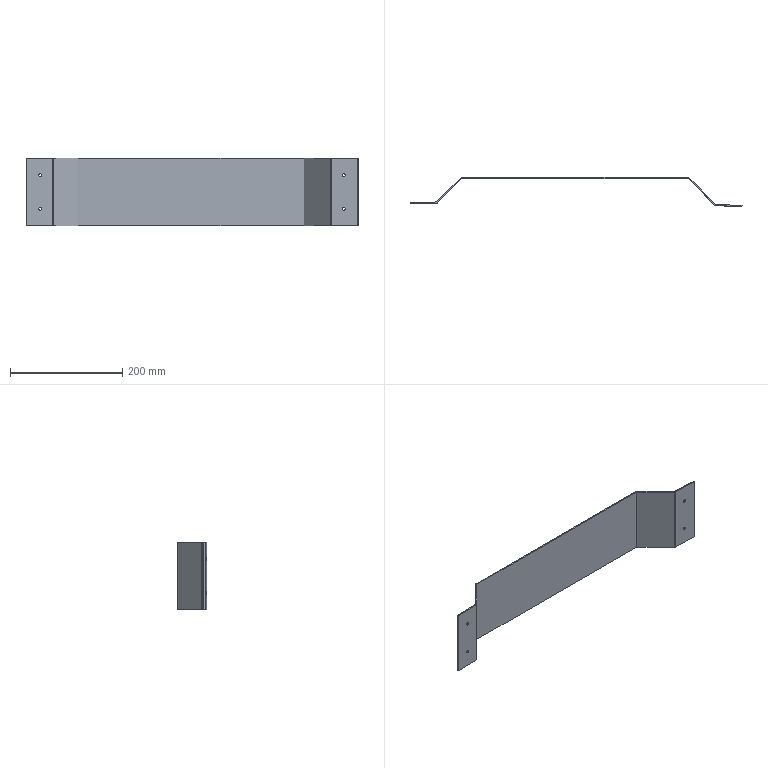Part | STEP file | Assembly TS-S02 | 1 solid | 46 faces | box 590.266 x 52.135 x 120 mm | volume 150616 mm3 | plane 30 | cylinder 16 | commonest cylinder face diameters 5 x8 0.4 x4 4.4 x4